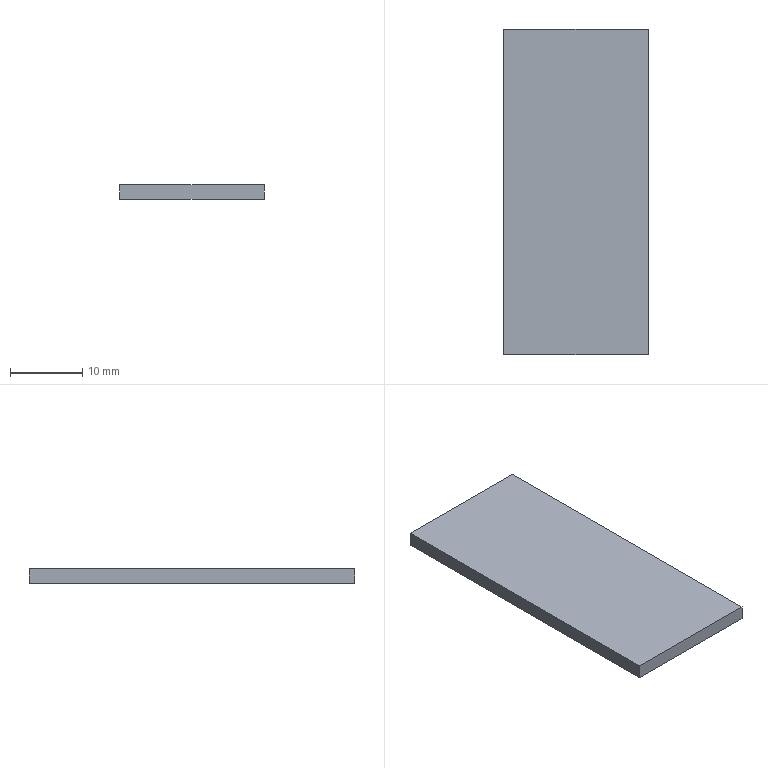Part | STEP file | Front Plate-1 | 1 solid | 6 faces | box 20 x 45 x 2 mm | volume 1800 mm3 | plane 6
STEP:
#1=CARTESIAN_POINT('',(20.,0.,-2.));
#2=VERTEX_POINT('',#1);
#3=CARTESIAN_POINT('',(0.,0.,-2.));
#4=VERTEX_POINT('',#3);
#5=CARTESIAN_POINT('',(0.,0.,-2.));
#6=DIRECTION('',(-1.,0.,0.));
#7=VECTOR('',#6,1000.);
#8=LINE('',#5,#7);
#9=EDGE_CURVE('',#2,#4,#8,.T.);
#10=ORIENTED_EDGE('',*,*,#9,.F.);
#11=CARTESIAN_POINT('',(20.,-45.,-2.));
#12=VERTEX_POINT('',#11);
#13=CARTESIAN_POINT('',(20.,0.,-2.));
#14=DIRECTION('',(0.,1.,0.));
#15=VECTOR('',#14,1000.);
#16=LINE('',#13,#15);
#17=EDGE_CURVE('',#12,#2,#16,.T.);
#18=ORIENTED_EDGE('',*,*,#17,.F.);
#19=CARTESIAN_POINT('',(0.,-45.,-2.));
#20=VERTEX_POINT('',#19);
#21=CARTESIAN_POINT('',(0.,-45.,-2.));
#22=DIRECTION('',(1.,0.,0.));
#23=VECTOR('',#22,1000.);
#24=LINE('',#21,#23);
#25=EDGE_CURVE('',#20,#12,#24,.T.);
#26=ORIENTED_EDGE('',*,*,#25,.F.);
#27=CARTESIAN_POINT('',(0.,0.,-2.));
#28=DIRECTION('',(0.,-1.,0.));
#29=VECTOR('',#28,1000.);
#30=LINE('',#27,#29);
#31=EDGE_CURVE('',#4,#20,#30,.T.);
#32=ORIENTED_EDGE('',*,*,#31,.F.);
#33=EDGE_LOOP('',(#10,#18,#26,#32));
#34=FACE_OUTER_BOUND('',#33,.T.);
#35=CARTESIAN_POINT('',(0.,0.,-2.));
#36=DIRECTION('',(0.,0.,1.));
#37=DIRECTION('',(1.,0.,0.));
#38=AXIS2_PLACEMENT_3D('',#35,#36,#37);
#39=PLANE('',#38);
#40=ADVANCED_FACE('',(#34),#39,.F.);
#41=ORIENTED_EDGE('',*,*,#31,.T.);
#42=CARTESIAN_POINT('',(0.,-45.,0.));
#43=VERTEX_POINT('',#42);
#44=CARTESIAN_POINT('',(0.,-45.,-2.));
#45=DIRECTION('',(0.,0.,1.));
#46=VECTOR('',#45,1000.);
#47=LINE('',#44,#46);
#48=EDGE_CURVE('',#20,#43,#47,.T.);
#49=ORIENTED_EDGE('',*,*,#48,.T.);
#50=CARTESIAN_POINT('',(0.,0.,0.));
#51=VERTEX_POINT('',#50);
#52=CARTESIAN_POINT('',(0.,0.,0.));
#53=DIRECTION('',(0.,1.,0.));
#54=VECTOR('',#53,1000.);
#55=LINE('',#52,#54);
#56=EDGE_CURVE('',#43,#51,#55,.T.);
#57=ORIENTED_EDGE('',*,*,#56,.T.);
#58=CARTESIAN_POINT('',(0.,0.,-2.));
#59=DIRECTION('',(0.,0.,-1.));
#60=VECTOR('',#59,1000.);
#61=LINE('',#58,#60);
#62=EDGE_CURVE('',#51,#4,#61,.T.);
#63=ORIENTED_EDGE('',*,*,#62,.T.);
#64=EDGE_LOOP('',(#41,#49,#57,#63));
#65=FACE_OUTER_BOUND('',#64,.T.);
#66=CARTESIAN_POINT('',(0.,0.,-2.));
#67=DIRECTION('',(-1.,0.,0.));
#68=DIRECTION('',(0.,-1.,0.));
#69=AXIS2_PLACEMENT_3D('',#66,#67,#68);
#70=PLANE('',#69);
#71=ADVANCED_FACE('',(#65),#70,.T.);
#72=ORIENTED_EDGE('',*,*,#9,.T.);
#73=ORIENTED_EDGE('',*,*,#62,.F.);
#74=CARTESIAN_POINT('',(20.,0.,0.));
#75=VERTEX_POINT('',#74);
#76=CARTESIAN_POINT('',(0.,0.,0.));
#77=DIRECTION('',(1.,0.,0.));
#78=VECTOR('',#77,1000.);
#79=LINE('',#76,#78);
#80=EDGE_CURVE('',#51,#75,#79,.T.);
#81=ORIENTED_EDGE('',*,*,#80,.T.);
#82=CARTESIAN_POINT('',(20.,0.,-2.));
#83=DIRECTION('',(0.,0.,-1.));
#84=VECTOR('',#83,1000.);
#85=LINE('',#82,#84);
#86=EDGE_CURVE('',#75,#2,#85,.T.);
#87=ORIENTED_EDGE('',*,*,#86,.T.);
#88=EDGE_LOOP('',(#72,#73,#81,#87));
#89=FACE_OUTER_BOUND('',#88,.T.);
#90=CARTESIAN_POINT('',(0.,0.,-2.));
#91=DIRECTION('',(0.,1.,0.));
#92=DIRECTION('',(0.,0.,1.));
#93=AXIS2_PLACEMENT_3D('',#90,#91,#92);
#94=PLANE('',#93);
#95=ADVANCED_FACE('',(#89),#94,.T.);
#96=ORIENTED_EDGE('',*,*,#17,.T.);
#97=ORIENTED_EDGE('',*,*,#86,.F.);
#98=CARTESIAN_POINT('',(20.,-45.,0.));
#99=VERTEX_POINT('',#98);
#100=CARTESIAN_POINT('',(20.,0.,0.));
#101=DIRECTION('',(0.,-1.,0.));
#102=VECTOR('',#101,1000.);
#103=LINE('',#100,#102);
#104=EDGE_CURVE('',#75,#99,#103,.T.);
#105=ORIENTED_EDGE('',*,*,#104,.T.);
#106=CARTESIAN_POINT('',(20.,-45.,-2.));
#107=DIRECTION('',(0.,0.,-1.));
#108=VECTOR('',#107,1000.);
#109=LINE('',#106,#108);
#110=EDGE_CURVE('',#99,#12,#109,.T.);
#111=ORIENTED_EDGE('',*,*,#110,.T.);
#112=EDGE_LOOP('',(#96,#97,#105,#111));
#113=FACE_OUTER_BOUND('',#112,.T.);
#114=CARTESIAN_POINT('',(20.,0.,-2.));
#115=DIRECTION('',(1.,0.,0.));
#116=DIRECTION('',(0.,1.,0.));
#117=AXIS2_PLACEMENT_3D('',#114,#115,#116);
#118=PLANE('',#117);
#119=ADVANCED_FACE('',(#113),#118,.T.);
#120=ORIENTED_EDGE('',*,*,#25,.T.);
#121=ORIENTED_EDGE('',*,*,#110,.F.);
#122=CARTESIAN_POINT('',(0.,-45.,0.));
#123=DIRECTION('',(-1.,0.,0.));
#124=VECTOR('',#123,1000.);
#125=LINE('',#122,#124);
#126=EDGE_CURVE('',#99,#43,#125,.T.);
#127=ORIENTED_EDGE('',*,*,#126,.T.);
#128=ORIENTED_EDGE('',*,*,#48,.F.);
#129=EDGE_LOOP('',(#120,#121,#127,#128));
#130=FACE_OUTER_BOUND('',#129,.T.);
#131=CARTESIAN_POINT('',(0.,-45.,-2.));
#132=DIRECTION('',(0.,-1.,0.));
#133=DIRECTION('',(0.,0.,-1.));
#134=AXIS2_PLACEMENT_3D('',#131,#132,#133);
#135=PLANE('',#134);
#136=ADVANCED_FACE('',(#130),#135,.T.);
#137=ORIENTED_EDGE('',*,*,#104,.F.);
#138=ORIENTED_EDGE('',*,*,#80,.F.);
#139=ORIENTED_EDGE('',*,*,#56,.F.);
#140=ORIENTED_EDGE('',*,*,#126,.F.);
#141=EDGE_LOOP('',(#137,#138,#139,#140));
#142=FACE_OUTER_BOUND('',#141,.T.);
#143=CARTESIAN_POINT('',(0.,0.,0.));
#144=DIRECTION('',(0.,0.,1.));
#145=DIRECTION('',(1.,0.,0.));
#146=AXIS2_PLACEMENT_3D('',#143,#144,#145);
#147=PLANE('',#146);
#148=ADVANCED_FACE('',(#142),#147,.T.);
#149=CLOSED_SHELL('',(#40,#71,#95,#119,#136,#148));
#150=MANIFOLD_SOLID_BREP('',#149);
#151=CARTESIAN_POINT('',(0.,0.,0.));
#152=DIRECTION('',(0.,0.,1.));
#153=DIRECTION('',(1.,0.,0.));
#154=AXIS2_PLACEMENT_3D('',#151,#152,#153);
#155=(LENGTH_UNIT()NAMED_UNIT(*)SI_UNIT(.MILLI.,.METRE.));
#156=UNCERTAINTY_MEASURE_WITH_UNIT(LENGTH_MEASURE(0.00001),#155,'','');
#157=(NAMED_UNIT(*)PLANE_ANGLE_UNIT()SI_UNIT($,.RADIAN.));
#158=(NAMED_UNIT(*)SI_UNIT($,.STERADIAN.)SOLID_ANGLE_UNIT());
#159=(GEOMETRIC_REPRESENTATION_CONTEXT(3)GLOBAL_UNCERTAINTY_ASSIGNED_CONTEXT((#156))GLOBAL_UNIT_ASSIGNED_CONTEXT((#155,#157,#158))REPRESENTATION_CONTEXT('',''));
#160=ADVANCED_BREP_SHAPE_REPRESENTATION('',(#150,#154),#159);